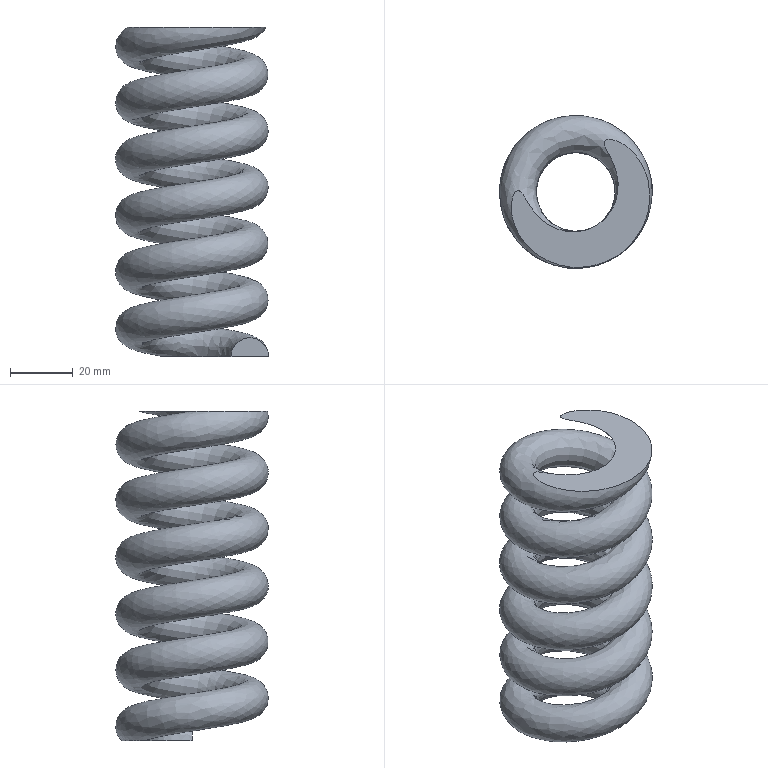Part | NX | features solid 2 | 1 solid | 4 faces | box 48.883 x 48.763 x 105 mm | volume 73970 mm3 | plane 3 | spline 1